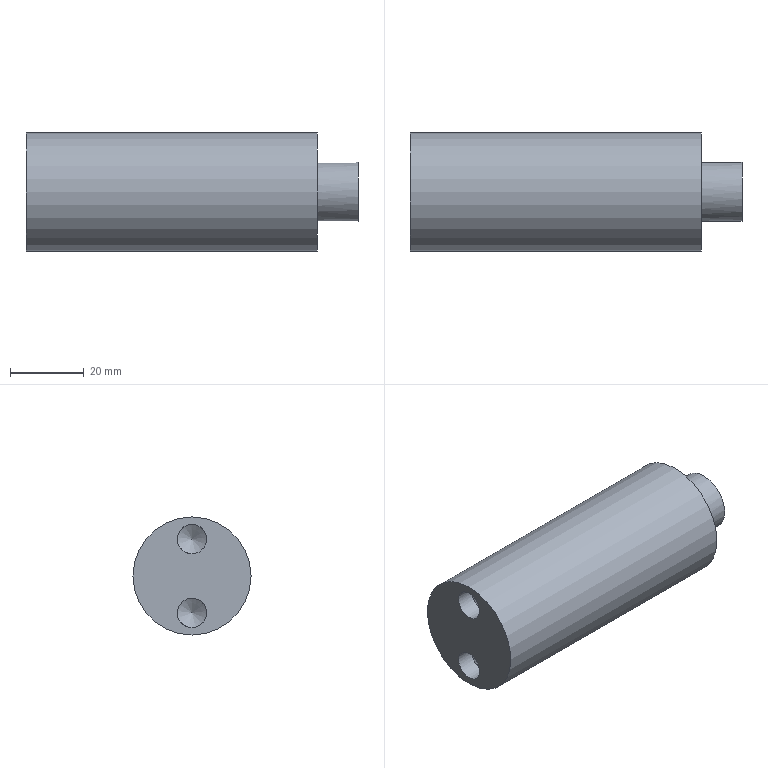Part | NX | features solid 2 | 1 solid | 9 faces | box 90 x 32 x 32 mm | volume 65164 mm3 | cylinder 4 | plane 3 | cone 2 | commonest cylinder face diameters 8 x2 16 x1 32 x1
STEP:
#1=CARTESIAN_POINT('',(968.701,-207.8,188.));
#2=VERTEX_POINT('',#1);
#3=CARTESIAN_POINT('',(968.701,-215.8,188.));
#4=DIRECTION('',(1.,0.,0.));
#5=DIRECTION('',(0.,1.,0.));
#6=AXIS2_PLACEMENT_3D('',#3,#4,#5);
#7=CIRCLE('',#6,8.);
#8=EDGE_CURVE('',#2,#2,#7,.F.);
#9=ORIENTED_EDGE('',*,*,#8,.T.);
#10=EDGE_LOOP('',(#9));
#11=FACE_BOUND('',#10,.T.);
#12=CARTESIAN_POINT('',(968.701,-199.8,188.));
#13=VERTEX_POINT('',#12);
#14=CARTESIAN_POINT('',(968.701,-215.8,188.));
#15=DIRECTION('',(1.,0.,0.));
#16=DIRECTION('',(0.,1.,0.));
#17=AXIS2_PLACEMENT_3D('',#14,#15,#16);
#18=CIRCLE('',#17,16.);
#19=EDGE_CURVE('',#13,#13,#18,.T.);
#20=ORIENTED_EDGE('',*,*,#19,.T.);
#21=EDGE_LOOP('',(#20));
#22=FACE_BOUND('',#21,.T.);
#23=CARTESIAN_POINT('',(968.701,-215.8,188.));
#24=DIRECTION('',(1.,0.,0.));
#25=DIRECTION('',(0.,0.,-1.));
#26=AXIS2_PLACEMENT_3D('',#23,#24,#25);
#27=PLANE('',#26);
#28=ADVANCED_FACE('',(#11,#22),#27,.T.);
#29=CARTESIAN_POINT('',(889.701,-211.8,198.));
#30=VERTEX_POINT('',#29);
#31=CARTESIAN_POINT('',(889.701,-215.8,198.));
#32=DIRECTION('',(-1.,0.,0.));
#33=DIRECTION('',(0.,1.,0.));
#34=AXIS2_PLACEMENT_3D('',#31,#32,#33);
#35=CIRCLE('',#34,4.);
#36=EDGE_CURVE('',#30,#30,#35,.T.);
#37=ORIENTED_EDGE('',*,*,#36,.F.);
#38=EDGE_LOOP('',(#37));
#39=FACE_BOUND('',#38,.T.);
#40=CARTESIAN_POINT('',(889.701,-211.8,178.));
#41=VERTEX_POINT('',#40);
#42=CARTESIAN_POINT('',(889.701,-215.8,178.));
#43=DIRECTION('',(-1.,0.,0.));
#44=DIRECTION('',(0.,1.,0.));
#45=AXIS2_PLACEMENT_3D('',#42,#43,#44);
#46=CIRCLE('',#45,4.);
#47=EDGE_CURVE('',#41,#41,#46,.T.);
#48=ORIENTED_EDGE('',*,*,#47,.F.);
#49=EDGE_LOOP('',(#48));
#50=FACE_BOUND('',#49,.T.);
#51=CARTESIAN_POINT('',(889.701,-215.8,172.));
#52=VERTEX_POINT('',#51);
#53=CARTESIAN_POINT('',(889.701,-215.8,188.));
#54=DIRECTION('',(-1.,0.,0.));
#55=DIRECTION('',(0.,0.,-1.));
#56=AXIS2_PLACEMENT_3D('',#53,#54,#55);
#57=CIRCLE('',#56,16.);
#58=EDGE_CURVE('',#52,#52,#57,.T.);
#59=ORIENTED_EDGE('',*,*,#58,.T.);
#60=EDGE_LOOP('',(#59));
#61=FACE_BOUND('',#60,.T.);
#62=CARTESIAN_POINT('',(889.701,-215.8,188.));
#63=DIRECTION('',(-1.,0.,0.));
#64=DIRECTION('',(0.,0.,1.));
#65=AXIS2_PLACEMENT_3D('',#62,#63,#64);
#66=PLANE('',#65);
#67=ADVANCED_FACE('',(#39,#50,#61),#66,.T.);
#68=ORIENTED_EDGE('',*,*,#19,.F.);
#69=EDGE_LOOP('',(#68));
#70=FACE_BOUND('',#69,.T.);
#71=ORIENTED_EDGE('',*,*,#58,.F.);
#72=EDGE_LOOP('',(#71));
#73=FACE_BOUND('',#72,.T.);
#74=CARTESIAN_POINT('',(879.701,-215.8,188.));
#75=DIRECTION('',(1.,0.,0.));
#76=DIRECTION('',(0.,0.,-1.));
#77=AXIS2_PLACEMENT_3D('',#74,#75,#76);
#78=CYLINDRICAL_SURFACE('',#77,16.);
#79=ADVANCED_FACE('',(#70,#73),#78,.T.);
#80=CARTESIAN_POINT('',(979.701,-215.8,196.));
#81=VERTEX_POINT('',#80);
#82=CARTESIAN_POINT('',(979.701,-215.8,188.));
#83=DIRECTION('',(1.,0.,0.));
#84=DIRECTION('',(0.,0.,1.));
#85=AXIS2_PLACEMENT_3D('',#82,#83,#84);
#86=CIRCLE('',#85,8.);
#87=EDGE_CURVE('',#81,#81,#86,.F.);
#88=ORIENTED_EDGE('',*,*,#87,.F.);
#89=EDGE_LOOP('',(#88));
#90=FACE_BOUND('',#89,.T.);
#91=CARTESIAN_POINT('',(979.701,-215.8,188.));
#92=DIRECTION('',(1.,0.,0.));
#93=DIRECTION('',(0.,0.,-1.));
#94=AXIS2_PLACEMENT_3D('',#91,#92,#93);
#95=PLANE('',#94);
#96=ADVANCED_FACE('',(#90),#95,.T.);
#97=ORIENTED_EDGE('',*,*,#87,.T.);
#98=EDGE_LOOP('',(#97));
#99=FACE_BOUND('',#98,.T.);
#100=ORIENTED_EDGE('',*,*,#8,.F.);
#101=EDGE_LOOP('',(#100));
#102=FACE_BOUND('',#101,.T.);
#103=CARTESIAN_POINT('',(1051.701,-215.8,188.));
#104=DIRECTION('',(1.,0.,0.));
#105=DIRECTION('',(0.,0.,-1.));
#106=AXIS2_PLACEMENT_3D('',#103,#104,#105);
#107=CYLINDRICAL_SURFACE('',#106,8.);
#108=ADVANCED_FACE('',(#99,#102),#107,.T.);
#109=CARTESIAN_POINT('',(894.701,-215.8,174.));
#110=VERTEX_POINT('',#109);
#111=CARTESIAN_POINT('',(894.701,-215.8,178.));
#112=DIRECTION('',(-1.,0.,0.));
#113=DIRECTION('',(0.,0.,-1.));
#114=AXIS2_PLACEMENT_3D('',#111,#112,#113);
#115=CIRCLE('',#114,4.);
#116=EDGE_CURVE('',#110,#110,#115,.T.);
#117=ORIENTED_EDGE('',*,*,#116,.T.);
#118=EDGE_LOOP('',(#117));
#119=FACE_BOUND('',#118,.T.);
#120=CARTESIAN_POINT('',(897.104,-215.8,178.));
#121=VERTEX_POINT('',#120);
#122=VERTEX_LOOP('',#121);
#123=FACE_BOUND('',#122,.T.);
#124=CARTESIAN_POINT('',(894.701,-215.8,178.));
#125=DIRECTION('',(-1.,0.,0.));
#126=DIRECTION('',(0.,0.,1.));
#127=AXIS2_PLACEMENT_3D('',#124,#125,#126);
#128=CONICAL_SURFACE('',#127,4.,1.03);
#129=ADVANCED_FACE('',(#119,#123),#128,.F.);
#130=ORIENTED_EDGE('',*,*,#116,.F.);
#131=EDGE_LOOP('',(#130));
#132=FACE_BOUND('',#131,.T.);
#133=ORIENTED_EDGE('',*,*,#47,.T.);
#134=EDGE_LOOP('',(#133));
#135=FACE_BOUND('',#134,.T.);
#136=CARTESIAN_POINT('',(879.701,-215.8,178.));
#137=DIRECTION('',(1.,0.,0.));
#138=DIRECTION('',(0.,0.,-1.));
#139=AXIS2_PLACEMENT_3D('',#136,#137,#138);
#140=CYLINDRICAL_SURFACE('',#139,4.);
#141=ADVANCED_FACE('',(#132,#135),#140,.F.);
#142=CARTESIAN_POINT('',(894.701,-215.8,194.));
#143=VERTEX_POINT('',#142);
#144=CARTESIAN_POINT('',(894.701,-215.8,198.));
#145=DIRECTION('',(-1.,0.,0.));
#146=DIRECTION('',(0.,0.,-1.));
#147=AXIS2_PLACEMENT_3D('',#144,#145,#146);
#148=CIRCLE('',#147,4.);
#149=EDGE_CURVE('',#143,#143,#148,.T.);
#150=ORIENTED_EDGE('',*,*,#149,.T.);
#151=EDGE_LOOP('',(#150));
#152=FACE_BOUND('',#151,.T.);
#153=CARTESIAN_POINT('',(897.104,-215.8,198.));
#154=VERTEX_POINT('',#153);
#155=VERTEX_LOOP('',#154);
#156=FACE_BOUND('',#155,.T.);
#157=CARTESIAN_POINT('',(894.701,-215.8,198.));
#158=DIRECTION('',(-1.,0.,0.));
#159=DIRECTION('',(0.,0.,1.));
#160=AXIS2_PLACEMENT_3D('',#157,#158,#159);
#161=CONICAL_SURFACE('',#160,4.,1.03);
#162=ADVANCED_FACE('',(#152,#156),#161,.F.);
#163=ORIENTED_EDGE('',*,*,#149,.F.);
#164=EDGE_LOOP('',(#163));
#165=FACE_BOUND('',#164,.T.);
#166=ORIENTED_EDGE('',*,*,#36,.T.);
#167=EDGE_LOOP('',(#166));
#168=FACE_BOUND('',#167,.T.);
#169=CARTESIAN_POINT('',(879.701,-215.8,198.));
#170=DIRECTION('',(1.,0.,0.));
#171=DIRECTION('',(0.,0.,-1.));
#172=AXIS2_PLACEMENT_3D('',#169,#170,#171);
#173=CYLINDRICAL_SURFACE('',#172,4.);
#174=ADVANCED_FACE('',(#165,#168),#173,.F.);
#175=CLOSED_SHELL('',(#28,#67,#79,#96,#108,#129,#141,#162,#174));
#176=MANIFOLD_SOLID_BREP('',#175);
#177=(LENGTH_UNIT()NAMED_UNIT(*)SI_UNIT(.MILLI.,.METRE.));
#178=UNCERTAINTY_MEASURE_WITH_UNIT(LENGTH_MEASURE(0.00001),#177,'','');
#179=(NAMED_UNIT(*)PLANE_ANGLE_UNIT()SI_UNIT($,.RADIAN.));
#180=(NAMED_UNIT(*)SI_UNIT($,.STERADIAN.)SOLID_ANGLE_UNIT());
#181=(GEOMETRIC_REPRESENTATION_CONTEXT(3)GLOBAL_UNCERTAINTY_ASSIGNED_CONTEXT((#178))GLOBAL_UNIT_ASSIGNED_CONTEXT((#177,#179,#180))REPRESENTATION_CONTEXT('',''));
#182=ADVANCED_BREP_SHAPE_REPRESENTATION('',(#176),#181);